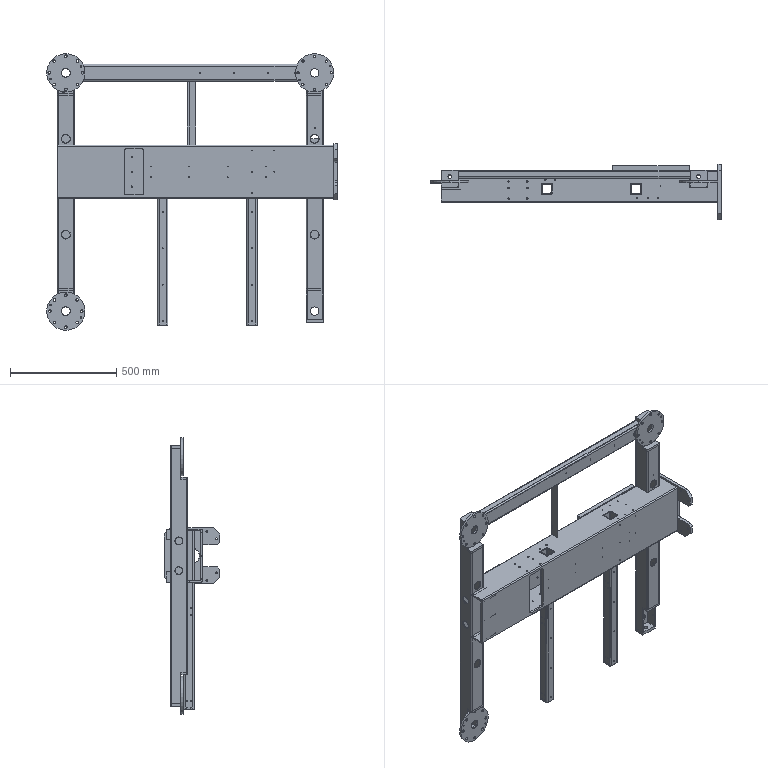Part | SolidWorks | 21 solids | 814 faces | box 1365 x 260 x 1300 mm | volume 14682038 mm3 | cylinder 543 | plane 205 | cone 66 | commonest cylinder face diameters 5 x118 4.2 x88 6.8 x52 8.5 x48 10 x47 12 x32